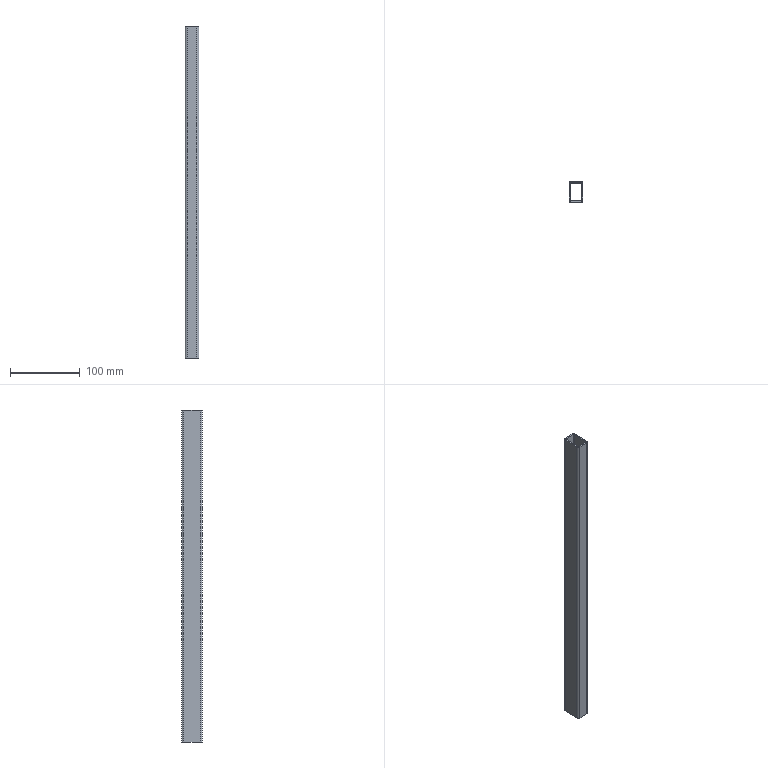Part | STEP file | DIN EN 10305-5 - 35 x 20 x 2  - 454 | 1 solid | 18 faces | box 20 x 30 x 475 mm | volume 84138 mm3 | plane 10 | cylinder 8 | commonest cylinder face diameters 2 x4 6 x4
STEP:
#1=CARTESIAN_POINT('',(0.,0.,0.));
#2=DIRECTION('',(0.,0.,1.));
#3=DIRECTION('',(1.,0.,0.));
#4=AXIS2_PLACEMENT_3D('',#1,#2,#3);
#5=CARTESIAN_POINT('',(-7.,-13.,475.));
#6=VERTEX_POINT('',#5);
#7=CARTESIAN_POINT('',(7.,-13.,475.));
#8=VERTEX_POINT('',#7);
#9=CARTESIAN_POINT('',(3.5,-13.,475.));
#10=DIRECTION('',(1.,0.,0.));
#11=VECTOR('',#10,1.);
#12=LINE('',#9,#11);
#13=CARTESIAN_POINT('',(7.,-13.,0.));
#14=DIRECTION('',(0.,-1.,0.));
#15=DIRECTION('',(0.,0.,-1.));
#16=AXIS2_PLACEMENT_3D('',#13,#14,#15);
#17=PLANE('',#16);
#18=CARTESIAN_POINT('',(-475.,-3.5));
#19=DIRECTION('',(0.,1.));
#20=VECTOR('',#19,1.);
#21=LINE('',#18,#20);
#22=(GEOMETRIC_REPRESENTATION_CONTEXT(2)PARAMETRIC_REPRESENTATION_CONTEXT()REPRESENTATION_CONTEXT('',''));
#23=DEFINITIONAL_REPRESENTATION('',(#21),#22);
#24=PCURVE('',#17,#23);
#25=CARTESIAN_POINT('',(0.,0.,475.));
#26=DIRECTION('',(0.,0.,1.));
#27=DIRECTION('',(1.,0.,0.));
#28=AXIS2_PLACEMENT_3D('',#25,#26,#27);
#29=PLANE('',#28);
#30=CARTESIAN_POINT('',(3.5,-13.));
#31=DIRECTION('',(1.,0.));
#32=VECTOR('',#31,1.);
#33=LINE('',#30,#32);
#34=(GEOMETRIC_REPRESENTATION_CONTEXT(2)PARAMETRIC_REPRESENTATION_CONTEXT()REPRESENTATION_CONTEXT('',''));
#35=DEFINITIONAL_REPRESENTATION('',(#33),#34);
#36=PCURVE('',#29,#35);
#37=SURFACE_CURVE('',#12,(#24,#36),.PCURVE_S1.);
#38=EDGE_CURVE('',#6,#8,#37,.T.);
#39=ORIENTED_EDGE('',*,*,#38,.T.);
#40=CARTESIAN_POINT('',(7.,-13.,0.));
#41=VERTEX_POINT('',#40);
#42=CARTESIAN_POINT('',(7.,-13.,0.));
#43=DIRECTION('',(0.,0.,1.));
#44=VECTOR('',#43,1.);
#45=LINE('',#42,#44);
#46=CARTESIAN_POINT('',(0.,0.));
#47=DIRECTION('',(-1.,0.));
#48=VECTOR('',#47,1.);
#49=LINE('',#46,#48);
#50=(GEOMETRIC_REPRESENTATION_CONTEXT(2)PARAMETRIC_REPRESENTATION_CONTEXT()REPRESENTATION_CONTEXT('',''));
#51=DEFINITIONAL_REPRESENTATION('',(#49),#50);
#52=PCURVE('',#17,#51);
#53=CARTESIAN_POINT('',(7.,-12.,0.));
#54=DIRECTION('',(0.,0.,1.));
#55=DIRECTION('',(0.,1.,0.));
#56=AXIS2_PLACEMENT_3D('',#53,#54,#55);
#57=CYLINDRICAL_SURFACE('',#56,1.);
#58=CARTESIAN_POINT('',(3.142,0.));
#59=DIRECTION('',(0.,1.));
#60=VECTOR('',#59,1.);
#61=LINE('',#58,#60);
#62=(GEOMETRIC_REPRESENTATION_CONTEXT(2)PARAMETRIC_REPRESENTATION_CONTEXT()REPRESENTATION_CONTEXT('',''));
#63=DEFINITIONAL_REPRESENTATION('',(#61),#62);
#64=PCURVE('',#57,#63);
#65=SURFACE_CURVE('',#45,(#52,#64),.PCURVE_S1.);
#66=EDGE_CURVE('',#41,#8,#65,.T.);
#67=ORIENTED_EDGE('',*,*,#66,.F.);
#68=CARTESIAN_POINT('',(-7.,-13.,0.));
#69=VERTEX_POINT('',#68);
#70=CARTESIAN_POINT('',(3.5,-13.,0.));
#71=DIRECTION('',(1.,0.,0.));
#72=VECTOR('',#71,1.);
#73=LINE('',#70,#72);
#74=CARTESIAN_POINT('',(0.,-3.5));
#75=DIRECTION('',(0.,1.));
#76=VECTOR('',#75,1.);
#77=LINE('',#74,#76);
#78=(GEOMETRIC_REPRESENTATION_CONTEXT(2)PARAMETRIC_REPRESENTATION_CONTEXT()REPRESENTATION_CONTEXT('',''));
#79=DEFINITIONAL_REPRESENTATION('',(#77),#78);
#80=PCURVE('',#17,#79);
#81=CARTESIAN_POINT('',(0.,0.,0.));
#82=DIRECTION('',(0.,0.,1.));
#83=DIRECTION('',(1.,0.,0.));
#84=AXIS2_PLACEMENT_3D('',#81,#82,#83);
#85=PLANE('',#84);
#86=CARTESIAN_POINT('',(3.5,-13.));
#87=DIRECTION('',(1.,0.));
#88=VECTOR('',#87,1.);
#89=LINE('',#86,#88);
#90=(GEOMETRIC_REPRESENTATION_CONTEXT(2)PARAMETRIC_REPRESENTATION_CONTEXT()REPRESENTATION_CONTEXT('',''));
#91=DEFINITIONAL_REPRESENTATION('',(#89),#90);
#92=PCURVE('',#85,#91);
#93=SURFACE_CURVE('',#73,(#80,#92),.PCURVE_S1.);
#94=EDGE_CURVE('',#69,#41,#93,.T.);
#95=ORIENTED_EDGE('',*,*,#94,.F.);
#96=CARTESIAN_POINT('',(-7.,-13.,0.));
#97=DIRECTION('',(0.,0.,1.));
#98=VECTOR('',#97,1.);
#99=LINE('',#96,#98);
#100=CARTESIAN_POINT('',(0.,-14.));
#101=DIRECTION('',(-1.,0.));
#102=VECTOR('',#101,1.);
#103=LINE('',#100,#102);
#104=(GEOMETRIC_REPRESENTATION_CONTEXT(2)PARAMETRIC_REPRESENTATION_CONTEXT()REPRESENTATION_CONTEXT('',''));
#105=DEFINITIONAL_REPRESENTATION('',(#103),#104);
#106=PCURVE('',#17,#105);
#107=CARTESIAN_POINT('',(-7.,-12.,0.));
#108=DIRECTION('',(0.,0.,1.));
#109=DIRECTION('',(1.,0.,0.));
#110=AXIS2_PLACEMENT_3D('',#107,#108,#109);
#111=CYLINDRICAL_SURFACE('',#110,1.);
#112=CARTESIAN_POINT('',(4.712,0.));
#113=DIRECTION('',(0.,1.));
#114=VECTOR('',#113,1.);
#115=LINE('',#112,#114);
#116=(GEOMETRIC_REPRESENTATION_CONTEXT(2)PARAMETRIC_REPRESENTATION_CONTEXT()REPRESENTATION_CONTEXT('',''));
#117=DEFINITIONAL_REPRESENTATION('',(#115),#116);
#118=PCURVE('',#111,#117);
#119=SURFACE_CURVE('',#99,(#106,#118),.PCURVE_S1.);
#120=EDGE_CURVE('',#69,#6,#119,.T.);
#121=ORIENTED_EDGE('',*,*,#120,.T.);
#122=EDGE_LOOP('',(#39,#67,#95,#121));
#123=FACE_BOUND('',#122,.T.);
#124=ADVANCED_FACE('',(#123),#17,.F.);
#125=ORIENTED_EDGE('',*,*,#66,.F.);
#126=CARTESIAN_POINT('',(8.,-12.,0.));
#127=VERTEX_POINT('',#126);
#128=CARTESIAN_POINT('',(7.,-12.,0.));
#129=DIRECTION('',(0.,0.,1.));
#130=DIRECTION('',(0.,1.,0.));
#131=AXIS2_PLACEMENT_3D('',#128,#129,#130);
#132=CIRCLE('',#131,1.);
#133=CARTESIAN_POINT('',(0.,0.));
#134=DIRECTION('',(1.,0.));
#135=VECTOR('',#134,1.);
#136=LINE('',#133,#135);
#137=(GEOMETRIC_REPRESENTATION_CONTEXT(2)PARAMETRIC_REPRESENTATION_CONTEXT()REPRESENTATION_CONTEXT('',''));
#138=DEFINITIONAL_REPRESENTATION('',(#136),#137);
#139=PCURVE('',#57,#138);
#140=CARTESIAN_POINT('',(7.,-12.));
#141=DIRECTION('',(0.,1.));
#142=AXIS2_PLACEMENT_2D('',#140,#141);
#143=CIRCLE('',#142,1.);
#144=(GEOMETRIC_REPRESENTATION_CONTEXT(2)PARAMETRIC_REPRESENTATION_CONTEXT()REPRESENTATION_CONTEXT('',''));
#145=DEFINITIONAL_REPRESENTATION('',(#143),#144);
#146=PCURVE('',#85,#145);
#147=SURFACE_CURVE('',#132,(#139,#146),.PCURVE_S1.);
#148=EDGE_CURVE('',#41,#127,#147,.T.);
#149=ORIENTED_EDGE('',*,*,#148,.T.);
#150=CARTESIAN_POINT('',(8.,-12.,475.));
#151=VERTEX_POINT('',#150);
#152=CARTESIAN_POINT('',(8.,-12.,0.));
#153=DIRECTION('',(0.,0.,1.));
#154=VECTOR('',#153,1.);
#155=LINE('',#152,#154);
#156=CARTESIAN_POINT('',(4.712,0.));
#157=DIRECTION('',(0.,1.));
#158=VECTOR('',#157,1.);
#159=LINE('',#156,#158);
#160=(GEOMETRIC_REPRESENTATION_CONTEXT(2)PARAMETRIC_REPRESENTATION_CONTEXT()REPRESENTATION_CONTEXT('',''));
#161=DEFINITIONAL_REPRESENTATION('',(#159),#160);
#162=PCURVE('',#57,#161);
#163=CARTESIAN_POINT('',(8.,12.,0.));
#164=DIRECTION('',(1.,0.,0.));
#165=DIRECTION('',(0.,0.,-1.));
#166=AXIS2_PLACEMENT_3D('',#163,#164,#165);
#167=PLANE('',#166);
#168=CARTESIAN_POINT('',(0.,-24.));
#169=DIRECTION('',(-1.,0.));
#170=VECTOR('',#169,1.);
#171=LINE('',#168,#170);
#172=(GEOMETRIC_REPRESENTATION_CONTEXT(2)PARAMETRIC_REPRESENTATION_CONTEXT()REPRESENTATION_CONTEXT('',''));
#173=DEFINITIONAL_REPRESENTATION('',(#171),#172);
#174=PCURVE('',#167,#173);
#175=SURFACE_CURVE('',#155,(#162,#174),.PCURVE_S1.);
#176=EDGE_CURVE('',#127,#151,#175,.T.);
#177=ORIENTED_EDGE('',*,*,#176,.T.);
#178=CARTESIAN_POINT('',(7.,-12.,475.));
#179=DIRECTION('',(0.,0.,1.));
#180=DIRECTION('',(0.,1.,0.));
#181=AXIS2_PLACEMENT_3D('',#178,#179,#180);
#182=CIRCLE('',#181,1.);
#183=CARTESIAN_POINT('',(0.,475.));
#184=DIRECTION('',(1.,0.));
#185=VECTOR('',#184,1.);
#186=LINE('',#183,#185);
#187=(GEOMETRIC_REPRESENTATION_CONTEXT(2)PARAMETRIC_REPRESENTATION_CONTEXT()REPRESENTATION_CONTEXT('',''));
#188=DEFINITIONAL_REPRESENTATION('',(#186),#187);
#189=PCURVE('',#57,#188);
#190=CARTESIAN_POINT('',(7.,-12.));
#191=DIRECTION('',(0.,1.));
#192=AXIS2_PLACEMENT_2D('',#190,#191);
#193=CIRCLE('',#192,1.);
#194=(GEOMETRIC_REPRESENTATION_CONTEXT(2)PARAMETRIC_REPRESENTATION_CONTEXT()REPRESENTATION_CONTEXT('',''));
#195=DEFINITIONAL_REPRESENTATION('',(#193),#194);
#196=PCURVE('',#29,#195);
#197=SURFACE_CURVE('',#182,(#189,#196),.PCURVE_S1.);
#198=EDGE_CURVE('',#8,#151,#197,.T.);
#199=ORIENTED_EDGE('',*,*,#198,.F.);
#200=EDGE_LOOP('',(#125,#149,#177,#199));
#201=FACE_BOUND('',#200,.F.);
#202=ADVANCED_FACE('',(#201),#57,.F.);
#203=CARTESIAN_POINT('',(8.,12.,475.));
#204=VERTEX_POINT('',#203);
#205=CARTESIAN_POINT('',(8.,6.,475.));
#206=DIRECTION('',(0.,1.,0.));
#207=VECTOR('',#206,1.);
#208=LINE('',#205,#207);
#209=CARTESIAN_POINT('',(-475.,-6.));
#210=DIRECTION('',(0.,1.));
#211=VECTOR('',#210,1.);
#212=LINE('',#209,#211);
#213=(GEOMETRIC_REPRESENTATION_CONTEXT(2)PARAMETRIC_REPRESENTATION_CONTEXT()REPRESENTATION_CONTEXT('',''));
#214=DEFINITIONAL_REPRESENTATION('',(#212),#213);
#215=PCURVE('',#167,#214);
#216=CARTESIAN_POINT('',(8.,6.));
#217=DIRECTION('',(0.,1.));
#218=VECTOR('',#217,1.);
#219=LINE('',#216,#218);
#220=(GEOMETRIC_REPRESENTATION_CONTEXT(2)PARAMETRIC_REPRESENTATION_CONTEXT()REPRESENTATION_CONTEXT('',''));
#221=DEFINITIONAL_REPRESENTATION('',(#219),#220);
#222=PCURVE('',#29,#221);
#223=SURFACE_CURVE('',#208,(#215,#222),.PCURVE_S1.);
#224=EDGE_CURVE('',#151,#204,#223,.T.);
#225=ORIENTED_EDGE('',*,*,#224,.T.);
#226=CARTESIAN_POINT('',(8.,12.,0.));
#227=VERTEX_POINT('',#226);
#228=CARTESIAN_POINT('',(8.,12.,0.));
#229=DIRECTION('',(0.,0.,1.));
#230=VECTOR('',#229,1.);
#231=LINE('',#228,#230);
#232=CARTESIAN_POINT('',(0.,0.));
#233=DIRECTION('',(-1.,0.));
#234=VECTOR('',#233,1.);
#235=LINE('',#232,#234);
#236=(GEOMETRIC_REPRESENTATION_CONTEXT(2)PARAMETRIC_REPRESENTATION_CONTEXT()REPRESENTATION_CONTEXT('',''));
#237=DEFINITIONAL_REPRESENTATION('',(#235),#236);
#238=PCURVE('',#167,#237);
#239=CARTESIAN_POINT('',(7.,12.,0.));
#240=DIRECTION('',(0.,0.,1.));
#241=DIRECTION('',(-1.,0.,0.));
#242=AXIS2_PLACEMENT_3D('',#239,#240,#241);
#243=CYLINDRICAL_SURFACE('',#242,1.);
#244=CARTESIAN_POINT('',(3.142,0.));
#245=DIRECTION('',(0.,1.));
#246=VECTOR('',#245,1.);
#247=LINE('',#244,#246);
#248=(GEOMETRIC_REPRESENTATION_CONTEXT(2)PARAMETRIC_REPRESENTATION_CONTEXT()REPRESENTATION_CONTEXT('',''));
#249=DEFINITIONAL_REPRESENTATION('',(#247),#248);
#250=PCURVE('',#243,#249);
#251=SURFACE_CURVE('',#231,(#238,#250),.PCURVE_S1.);
#252=EDGE_CURVE('',#227,#204,#251,.T.);
#253=ORIENTED_EDGE('',*,*,#252,.F.);
#254=CARTESIAN_POINT('',(8.,6.,0.));
#255=DIRECTION('',(0.,1.,0.));
#256=VECTOR('',#255,1.);
#257=LINE('',#254,#256);
#258=CARTESIAN_POINT('',(0.,-6.));
#259=DIRECTION('',(0.,1.));
#260=VECTOR('',#259,1.);
#261=LINE('',#258,#260);
#262=(GEOMETRIC_REPRESENTATION_CONTEXT(2)PARAMETRIC_REPRESENTATION_CONTEXT()REPRESENTATION_CONTEXT('',''));
#263=DEFINITIONAL_REPRESENTATION('',(#261),#262);
#264=PCURVE('',#167,#263);
#265=CARTESIAN_POINT('',(8.,6.));
#266=DIRECTION('',(0.,1.));
#267=VECTOR('',#266,1.);
#268=LINE('',#265,#267);
#269=(GEOMETRIC_REPRESENTATION_CONTEXT(2)PARAMETRIC_REPRESENTATION_CONTEXT()REPRESENTATION_CONTEXT('',''));
#270=DEFINITIONAL_REPRESENTATION('',(#268),#269);
#271=PCURVE('',#85,#270);
#272=SURFACE_CURVE('',#257,(#264,#271),.PCURVE_S1.);
#273=EDGE_CURVE('',#127,#227,#272,.T.);
#274=ORIENTED_EDGE('',*,*,#273,.F.);
#275=ORIENTED_EDGE('',*,*,#176,.T.);
#276=EDGE_LOOP('',(#225,#253,#274,#275));
#277=FACE_BOUND('',#276,.T.);
#278=ADVANCED_FACE('',(#277),#167,.F.);
#279=ORIENTED_EDGE('',*,*,#252,.F.);
#280=CARTESIAN_POINT('',(7.,13.,0.));
#281=VERTEX_POINT('',#280);
#282=CARTESIAN_POINT('',(7.,12.,0.));
#283=DIRECTION('',(0.,0.,1.));
#284=DIRECTION('',(-1.,0.,0.));
#285=AXIS2_PLACEMENT_3D('',#282,#283,#284);
#286=CIRCLE('',#285,1.);
#287=CARTESIAN_POINT('',(0.,0.));
#288=DIRECTION('',(1.,0.));
#289=VECTOR('',#288,1.);
#290=LINE('',#287,#289);
#291=(GEOMETRIC_REPRESENTATION_CONTEXT(2)PARAMETRIC_REPRESENTATION_CONTEXT()REPRESENTATION_CONTEXT('',''));
#292=DEFINITIONAL_REPRESENTATION('',(#290),#291);
#293=PCURVE('',#243,#292);
#294=CARTESIAN_POINT('',(7.,12.));
#295=DIRECTION('',(-1.,0.));
#296=AXIS2_PLACEMENT_2D('',#294,#295);
#297=CIRCLE('',#296,1.);
#298=(GEOMETRIC_REPRESENTATION_CONTEXT(2)PARAMETRIC_REPRESENTATION_CONTEXT()REPRESENTATION_CONTEXT('',''));
#299=DEFINITIONAL_REPRESENTATION('',(#297),#298);
#300=PCURVE('',#85,#299);
#301=SURFACE_CURVE('',#286,(#293,#300),.PCURVE_S1.);
#302=EDGE_CURVE('',#227,#281,#301,.T.);
#303=ORIENTED_EDGE('',*,*,#302,.T.);
#304=CARTESIAN_POINT('',(7.,13.,475.));
#305=VERTEX_POINT('',#304);
#306=CARTESIAN_POINT('',(7.,13.,0.));
#307=DIRECTION('',(0.,0.,1.));
#308=VECTOR('',#307,1.);
#309=LINE('',#306,#308);
#310=CARTESIAN_POINT('',(4.712,0.));
#311=DIRECTION('',(0.,1.));
#312=VECTOR('',#311,1.);
#313=LINE('',#310,#312);
#314=(GEOMETRIC_REPRESENTATION_CONTEXT(2)PARAMETRIC_REPRESENTATION_CONTEXT()REPRESENTATION_CONTEXT('',''));
#315=DEFINITIONAL_REPRESENTATION('',(#313),#314);
#316=PCURVE('',#243,#315);
#317=CARTESIAN_POINT('',(-7.,13.,0.));
#318=DIRECTION('',(0.,1.,0.));
#319=DIRECTION('',(0.,0.,1.));
#320=AXIS2_PLACEMENT_3D('',#317,#318,#319);
#321=PLANE('',#320);
#322=CARTESIAN_POINT('',(0.,14.));
#323=DIRECTION('',(1.,0.));
#324=VECTOR('',#323,1.);
#325=LINE('',#322,#324);
#326=(GEOMETRIC_REPRESENTATION_CONTEXT(2)PARAMETRIC_REPRESENTATION_CONTEXT()REPRESENTATION_CONTEXT('',''));
#327=DEFINITIONAL_REPRESENTATION('',(#325),#326);
#328=PCURVE('',#321,#327);
#329=SURFACE_CURVE('',#309,(#316,#328),.PCURVE_S1.);
#330=EDGE_CURVE('',#281,#305,#329,.T.);
#331=ORIENTED_EDGE('',*,*,#330,.T.);
#332=CARTESIAN_POINT('',(7.,12.,475.));
#333=DIRECTION('',(0.,0.,1.));
#334=DIRECTION('',(-1.,0.,0.));
#335=AXIS2_PLACEMENT_3D('',#332,#333,#334);
#336=CIRCLE('',#335,1.);
#337=CARTESIAN_POINT('',(0.,475.));
#338=DIRECTION('',(1.,0.));
#339=VECTOR('',#338,1.);
#340=LINE('',#337,#339);
#341=(GEOMETRIC_REPRESENTATION_CONTEXT(2)PARAMETRIC_REPRESENTATION_CONTEXT()REPRESENTATION_CONTEXT('',''));
#342=DEFINITIONAL_REPRESENTATION('',(#340),#341);
#343=PCURVE('',#243,#342);
#344=CARTESIAN_POINT('',(7.,12.));
#345=DIRECTION('',(-1.,0.));
#346=AXIS2_PLACEMENT_2D('',#344,#345);
#347=CIRCLE('',#346,1.);
#348=(GEOMETRIC_REPRESENTATION_CONTEXT(2)PARAMETRIC_REPRESENTATION_CONTEXT()REPRESENTATION_CONTEXT('',''));
#349=DEFINITIONAL_REPRESENTATION('',(#347),#348);
#350=PCURVE('',#29,#349);
#351=SURFACE_CURVE('',#336,(#343,#350),.PCURVE_S1.);
#352=EDGE_CURVE('',#204,#305,#351,.T.);
#353=ORIENTED_EDGE('',*,*,#352,.F.);
#354=EDGE_LOOP('',(#279,#303,#331,#353));
#355=FACE_BOUND('',#354,.F.);
#356=ADVANCED_FACE('',(#355),#243,.F.);
#357=CARTESIAN_POINT('',(10.,12.,475.));
#358=VERTEX_POINT('',#357);
#359=CARTESIAN_POINT('',(10.,-12.,475.));
#360=VERTEX_POINT('',#359);
#361=CARTESIAN_POINT('',(10.,6.,475.));
#362=DIRECTION('',(0.,-1.,0.));
#363=VECTOR('',#362,1.);
#364=LINE('',#361,#363);
#365=CARTESIAN_POINT('',(10.,12.,0.));
#366=DIRECTION('',(1.,0.,0.));
#367=DIRECTION('',(0.,0.,-1.));
#368=AXIS2_PLACEMENT_3D('',#365,#366,#367);
#369=PLANE('',#368);
#370=CARTESIAN_POINT('',(-475.,-6.));
#371=DIRECTION('',(0.,-1.));
#372=VECTOR('',#371,1.);
#373=LINE('',#370,#372);
#374=(GEOMETRIC_REPRESENTATION_CONTEXT(2)PARAMETRIC_REPRESENTATION_CONTEXT()REPRESENTATION_CONTEXT('',''));
#375=DEFINITIONAL_REPRESENTATION('',(#373),#374);
#376=PCURVE('',#369,#375);
#377=CARTESIAN_POINT('',(10.,6.));
#378=DIRECTION('',(0.,-1.));
#379=VECTOR('',#378,1.);
#380=LINE('',#377,#379);
#381=(GEOMETRIC_REPRESENTATION_CONTEXT(2)PARAMETRIC_REPRESENTATION_CONTEXT()REPRESENTATION_CONTEXT('',''));
#382=DEFINITIONAL_REPRESENTATION('',(#380),#381);
#383=PCURVE('',#29,#382);
#384=SURFACE_CURVE('',#364,(#376,#383),.PCURVE_S1.);
#385=EDGE_CURVE('',#358,#360,#384,.T.);
#386=ORIENTED_EDGE('',*,*,#385,.T.);
#387=CARTESIAN_POINT('',(10.,-12.,0.));
#388=VERTEX_POINT('',#387);
#389=CARTESIAN_POINT('',(10.,-12.,0.));
#390=DIRECTION('',(0.,0.,1.));
#391=VECTOR('',#390,1.);
#392=LINE('',#389,#391);
#393=CARTESIAN_POINT('',(0.,-24.));
#394=DIRECTION('',(-1.,0.));
#395=VECTOR('',#394,1.);
#396=LINE('',#393,#395);
#397=(GEOMETRIC_REPRESENTATION_CONTEXT(2)PARAMETRIC_REPRESENTATION_CONTEXT()REPRESENTATION_CONTEXT('',''));
#398=DEFINITIONAL_REPRESENTATION('',(#396),#397);
#399=PCURVE('',#369,#398);
#400=CARTESIAN_POINT('',(7.,-12.,0.));
#401=DIRECTION('',(0.,0.,1.));
#402=DIRECTION('',(0.,1.,0.));
#403=AXIS2_PLACEMENT_3D('',#400,#401,#402);
#404=CYLINDRICAL_SURFACE('',#403,3.);
#405=CARTESIAN_POINT('',(4.712,0.));
#406=DIRECTION('',(0.,1.));
#407=VECTOR('',#406,1.);
#408=LINE('',#405,#407);
#409=(GEOMETRIC_REPRESENTATION_CONTEXT(2)PARAMETRIC_REPRESENTATION_CONTEXT()REPRESENTATION_CONTEXT('',''));
#410=DEFINITIONAL_REPRESENTATION('',(#408),#409);
#411=PCURVE('',#404,#410);
#412=SURFACE_CURVE('',#392,(#399,#411),.PCURVE_S1.);
#413=EDGE_CURVE('',#388,#360,#412,.T.);
#414=ORIENTED_EDGE('',*,*,#413,.F.);
#415=CARTESIAN_POINT('',(10.,12.,0.));
#416=VERTEX_POINT('',#415);
#417=CARTESIAN_POINT('',(10.,6.,0.));
#418=DIRECTION('',(0.,-1.,0.));
#419=VECTOR('',#418,1.);
#420=LINE('',#417,#419);
#421=CARTESIAN_POINT('',(0.,-6.));
#422=DIRECTION('',(0.,-1.));
#423=VECTOR('',#422,1.);
#424=LINE('',#421,#423);
#425=(GEOMETRIC_REPRESENTATION_CONTEXT(2)PARAMETRIC_REPRESENTATION_CONTEXT()REPRESENTATION_CONTEXT('',''));
#426=DEFINITIONAL_REPRESENTATION('',(#424),#425);
#427=PCURVE('',#369,#426);
#428=CARTESIAN_POINT('',(10.,6.));
#429=DIRECTION('',(0.,-1.));
#430=VECTOR('',#429,1.);
#431=LINE('',#428,#430);
#432=(GEOMETRIC_REPRESENTATION_CONTEXT(2)PARAMETRIC_REPRESENTATION_CONTEXT()REPRESENTATION_CONTEXT('',''));
#433=DEFINITIONAL_REPRESENTATION('',(#431),#432);
#434=PCURVE('',#85,#433);
#435=SURFACE_CURVE('',#420,(#427,#434),.PCURVE_S1.);
#436=EDGE_CURVE('',#416,#388,#435,.T.);
#437=ORIENTED_EDGE('',*,*,#436,.F.);
#438=CARTESIAN_POINT('',(10.,12.,0.));
#439=DIRECTION('',(0.,0.,1.));
#440=VECTOR('',#439,1.);
#441=LINE('',#438,#440);
#442=CARTESIAN_POINT('',(0.,0.));
#443=DIRECTION('',(-1.,0.));
#444=VECTOR('',#443,1.);
#445=LINE('',#442,#444);
#446=(GEOMETRIC_REPRESENTATION_CONTEXT(2)PARAMETRIC_REPRESENTATION_CONTEXT()REPRESENTATION_CONTEXT('',''));
#447=DEFINITIONAL_REPRESENTATION('',(#445),#446);
#448=PCURVE('',#369,#447);
#449=CARTESIAN_POINT('',(7.,12.,0.));
#450=DIRECTION('',(0.,0.,1.));
#451=DIRECTION('',(-1.,0.,0.));
#452=AXIS2_PLACEMENT_3D('',#449,#450,#451);
#453=CYLINDRICAL_SURFACE('',#452,3.);
#454=CARTESIAN_POINT('',(3.142,0.));
#455=DIRECTION('',(0.,1.));
#456=VECTOR('',#455,1.);
#457=LINE('',#454,#456);
#458=(GEOMETRIC_REPRESENTATION_CONTEXT(2)PARAMETRIC_REPRESENTATION_CONTEXT()REPRESENTATION_CONTEXT('',''));
#459=DEFINITIONAL_REPRESENTATION('',(#457),#458);
#460=PCURVE('',#453,#459);
#461=SURFACE_CURVE('',#441,(#448,#460),.PCURVE_S1.);
#462=EDGE_CURVE('',#416,#358,#461,.T.);
#463=ORIENTED_EDGE('',*,*,#462,.T.);
#464=EDGE_LOOP('',(#386,#414,#437,#463));
#465=FACE_BOUND('',#464,.T.);
#466=ADVANCED_FACE('',(#465),#369,.T.);
#467=CARTESIAN_POINT('',(7.,-15.,475.));
#468=VERTEX_POINT('',#467);
#469=CARTESIAN_POINT('',(7.,-12.,475.));
#470=DIRECTION('',(0.,0.,-1.));
#471=DIRECTION('',(0.,1.,0.));
#472=AXIS2_PLACEMENT_3D('',#469,#470,#471);
#473=CIRCLE('',#472,3.);
#474=CARTESIAN_POINT('',(6.283,475.));
#475=DIRECTION('',(-1.,0.));
#476=VECTOR('',#475,1.);
#477=LINE('',#474,#476);
#478=(GEOMETRIC_REPRESENTATION_CONTEXT(2)PARAMETRIC_REPRESENTATION_CONTEXT()REPRESENTATION_CONTEXT('',''));
#479=DEFINITIONAL_REPRESENTATION('',(#477),#478);
#480=PCURVE('',#404,#479);
#481=CARTESIAN_POINT('',(7.,-9.));
#482=CARTESIAN_POINT('',(12.196,-9.));
#483=CARTESIAN_POINT('',(9.598,-13.5));
#484=CARTESIAN_POINT('',(7.,-18.));
#485=CARTESIAN_POINT('',(4.402,-13.5));
#486=CARTESIAN_POINT('',(1.804,-9.));
#487=CARTESIAN_POINT('',(7.,-9.));
#488=(BOUNDED_CURVE()B_SPLINE_CURVE(2,(#481,#482,#483,#484,#485,#486,#487),.UNSPECIFIED.,.T.,.F.)B_SPLINE_CURVE_WITH_KNOTS((1,2,2,2,2,1),(-2.094,0.,2.094,4.189,6.283,8.378),.UNSPECIFIED.)CURVE()GEOMETRIC_REPRESENTATION_ITEM()RATIONAL_B_SPLINE_CURVE((1.,0.5,1.,0.5,1.,0.5,1.))REPRESENTATION_ITEM(''));
#489=(GEOMETRIC_REPRESENTATION_CONTEXT(2)PARAMETRIC_REPRESENTATION_CONTEXT()REPRESENTATION_CONTEXT('',''));
#490=DEFINITIONAL_REPRESENTATION('',(#488),#489);
#491=PCURVE('',#29,#490);
#492=SURFACE_CURVE('',#473,(#480,#491),.PCURVE_S1.);
#493=EDGE_CURVE('',#360,#468,#492,.T.);
#494=ORIENTED_EDGE('',*,*,#493,.T.);
#495=CARTESIAN_POINT('',(7.,-15.,0.));
#496=VERTEX_POINT('',#495);
#497=CARTESIAN_POINT('',(7.,-15.,0.));
#498=DIRECTION('',(0.,0.,1.));
#499=VECTOR('',#498,1.);
#500=LINE('',#497,#499);
#501=CARTESIAN_POINT('',(3.142,0.));
#502=DIRECTION('',(0.,1.));
#503=VECTOR('',#502,1.);
#504=LINE('',#501,#503);
#505=(GEOMETRIC_REPRESENTATION_CONTEXT(2)PARAMETRIC_REPRESENTATION_CONTEXT()REPRESENTATION_CONTEXT('',''));
#506=DEFINITIONAL_REPRESENTATION('',(#504),#505);
#507=PCURVE('',#404,#506);
#508=CARTESIAN_POINT('',(7.,-15.,0.));
#509=DIRECTION('',(0.,-1.,0.));
#510=DIRECTION('',(0.,0.,-1.));
#511=AXIS2_PLACEMENT_3D('',#508,#509,#510);
#512=PLANE('',#511);
#513=CARTESIAN_POINT('',(0.,0.));
#514=DIRECTION('',(-1.,0.));
#515=VECTOR('',#514,1.);
#516=LINE('',#513,#515);
#517=(GEOMETRIC_REPRESENTATION_CONTEXT(2)PARAMETRIC_REPRESENTATION_CONTEXT()REPRESENTATION_CONTEXT('',''));
#518=DEFINITIONAL_REPRESENTATION('',(#516),#517);
#519=PCURVE('',#512,#518);
#520=SURFACE_CURVE('',#500,(#507,#519),.PCURVE_S1.);
#521=EDGE_CURVE('',#496,#468,#520,.T.);
#522=ORIENTED_EDGE('',*,*,#521,.F.);
#523=CARTESIAN_POINT('',(7.,-12.,0.));
#524=DIRECTION('',(0.,0.,-1.));
#525=DIRECTION('',(0.,1.,0.));
#526=AXIS2_PLACEMENT_3D('',#523,#524,#525);
#527=CIRCLE('',#526,3.);
#528=CARTESIAN_POINT('',(6.283,0.));
#529=DIRECTION('',(-1.,0.));
#530=VECTOR('',#529,1.);
#531=LINE('',#528,#530);
#532=(GEOMETRIC_REPRESENTATION_CONTEXT(2)PARAMETRIC_REPRESENTATION_CONTEXT()REPRESENTATION_CONTEXT('',''));
#533=DEFINITIONAL_REPRESENTATION('',(#531),#532);
#534=PCURVE('',#404,#533);
#535=CARTESIAN_POINT('',(7.,-9.));
#536=CARTESIAN_POINT('',(12.196,-9.));
#537=CARTESIAN_POINT('',(9.598,-13.5));
#538=CARTESIAN_POINT('',(7.,-18.));
#539=CARTESIAN_POINT('',(4.402,-13.5));
#540=CARTESIAN_POINT('',(1.804,-9.));
#541=CARTESIAN_POINT('',(7.,-9.));
#542=(BOUNDED_CURVE()B_SPLINE_CURVE(2,(#535,#536,#537,#538,#539,#540,#541),.UNSPECIFIED.,.T.,.F.)B_SPLINE_CURVE_WITH_KNOTS((1,2,2,2,2,1),(-2.094,0.,2.094,4.189,6.283,8.378),.UNSPECIFIED.)CURVE()GEOMETRIC_REPRESENTATION_ITEM()RATIONAL_B_SPLINE_CURVE((1.,0.5,1.,0.5,1.,0.5,1.))REPRESENTATION_ITEM(''));
#543=(GEOMETRIC_REPRESENTATION_CONTEXT(2)PARAMETRIC_REPRESENTATION_CONTEXT()REPRESENTATION_CONTEXT('',''));
#544=DEFINITIONAL_REPRESENTATION('',(#542),#543);
#545=PCURVE('',#85,#544);
#546=SURFACE_CURVE('',#527,(#534,#545),.PCURVE_S1.);
#547=EDGE_CURVE('',#388,#496,#546,.T.);
#548=ORIENTED_EDGE('',*,*,#547,.F.);
#549=ORIENTED_EDGE('',*,*,#413,.T.);
#550=EDGE_LOOP('',(#494,#522,#548,#549));
#551=FACE_BOUND('',#550,.T.);
#552=ADVANCED_FACE('',(#551),#404,.T.);
#553=CARTESIAN_POINT('',(-7.,-15.,475.));
#554=VERTEX_POINT('',#553);
#555=CARTESIAN_POINT('',(3.5,-15.,475.));
#556=DIRECTION('',(-1.,0.,0.));
#557=VECTOR('',#556,1.);
#558=LINE('',#555,#557);
#559=CARTESIAN_POINT('',(-475.,-3.5));
#560=DIRECTION('',(0.,-1.));
#561=VECTOR('',#560,1.);
#562=LINE('',#559,#561);
#563=(GEOMETRIC_REPRESENTATION_CONTEXT(2)PARAMETRIC_REPRESENTATION_CONTEXT()REPRESENTATION_CONTEXT('',''));
#564=DEFINITIONAL_REPRESENTATION('',(#562),#563);
#565=PCURVE('',#512,#564);
#566=CARTESIAN_POINT('',(3.5,-15.));
#567=DIRECTION('',(-1.,0.));
#568=VECTOR('',#567,1.);
#569=LINE('',#566,#568);
#570=(GEOMETRIC_REPRESENTATION_CONTEXT(2)PARAMETRIC_REPRESENTATION_CONTEXT()REPRESENTATION_CONTEXT('',''));
#571=DEFINITIONAL_REPRESENTATION('',(#569),#570);
#572=PCURVE('',#29,#571);
#573=SURFACE_CURVE('',#558,(#565,#572),.PCURVE_S1.);
#574=EDGE_CURVE('',#468,#554,#573,.T.);
#575=ORIENTED_EDGE('',*,*,#574,.T.);
#576=CARTESIAN_POINT('',(-7.,-15.,0.));
#577=VERTEX_POINT('',#576);
#578=CARTESIAN_POINT('',(-7.,-15.,0.));
#579=DIRECTION('',(0.,0.,1.));
#580=VECTOR('',#579,1.);
#581=LINE('',#578,#580);
#582=CARTESIAN_POINT('',(0.,-14.));
#583=DIRECTION('',(-1.,0.));
#584=VECTOR('',#583,1.);
#585=LINE('',#582,#584);
#586=(GEOMETRIC_REPRESENTATION_CONTEXT(2)PARAMETRIC_REPRESENTATION_CONTEXT()REPRESENTATION_CONTEXT('',''));
#587=DEFINITIONAL_REPRESENTATION('',(#585),#586);
#588=PCURVE('',#512,#587);
#589=CARTESIAN_POINT('',(-7.,-12.,0.));
#590=DIRECTION('',(0.,0.,1.));
#591=DIRECTION('',(1.,0.,0.));
#592=AXIS2_PLACEMENT_3D('',#589,#590,#591);
#593=CYLINDRICAL_SURFACE('',#592,3.);
#594=CARTESIAN_POINT('',(4.712,0.));
#595=DIRECTION('',(0.,1.));
#596=VECTOR('',#595,1.);
#597=LINE('',#594,#596);
#598=(GEOMETRIC_REPRESENTATION_CONTEXT(2)PARAMETRIC_REPRESENTATION_CONTEXT()REPRESENTATION_CONTEXT('',''));
#599=DEFINITIONAL_REPRESENTATION('',(#597),#598);
#600=PCURVE('',#593,#599);
#601=SURFACE_CURVE('',#581,(#588,#600),.PCURVE_S1.);
#602=EDGE_CURVE('',#577,#554,#601,.T.);
#603=ORIENTED_EDGE('',*,*,#602,.F.);
#604=CARTESIAN_POINT('',(3.5,-15.,0.));
#605=DIRECTION('',(-1.,0.,0.));
#606=VECTOR('',#605,1.);
#607=LINE('',#604,#606);
#608=CARTESIAN_POINT('',(0.,-3.5));
#609=DIRECTION('',(0.,-1.));
#610=VECTOR('',#609,1.);
#611=LINE('',#608,#610);
#612=(GEOMETRIC_REPRESENTATION_CONTEXT(2)PARAMETRIC_REPRESENTATION_CONTEXT()REPRESENTATION_CONTEXT('',''));
#613=DEFINITIONAL_REPRESENTATION('',(#611),#612);
#614=PCURVE('',#512,#613);
#615=CARTESIAN_POINT('',(3.5,-15.));
#616=DIRECTION('',(-1.,0.));
#617=VECTOR('',#616,1.);
#618=LINE('',#615,#617);
#619=(GEOMETRIC_REPRESENTATION_CONTEXT(2)PARAMETRIC_REPRESENTATION_CONTEXT()REPRESENTATION_CONTEXT('',''));
#620=DEFINITIONAL_REPRESENTATION('',(#618),#619);
#621=PCURVE('',#85,#620);
#622=SURFACE_CURVE('',#607,(#614,#621),.PCURVE_S1.);
#623=EDGE_CURVE('',#496,#577,#622,.T.);
#624=ORIENTED_EDGE('',*,*,#623,.F.);
#625=ORIENTED_EDGE('',*,*,#521,.T.);
#626=EDGE_LOOP('',(#575,#603,#624,#625));
#627=FACE_BOUND('',#626,.T.);
#628=ADVANCED_FACE('',(#627),#512,.T.);
#629=CARTESIAN_POINT('',(-10.,-12.,475.));
#630=VERTEX_POINT('',#629);
#631=CARTESIAN_POINT('',(-7.,-12.,475.));
#632=DIRECTION('',(0.,0.,-1.));
#633=DIRECTION('',(1.,0.,0.));
#634=AXIS2_PLACEMENT_3D('',#631,#632,#633);
#635=CIRCLE('',#634,3.);
#636=CARTESIAN_POINT('',(6.283,475.));
#637=DIRECTION('',(-1.,0.));
#638=VECTOR('',#637,1.);
#639=LINE('',#636,#638);
#640=(GEOMETRIC_REPRESENTATION_CONTEXT(2)PARAMETRIC_REPRESENTATION_CONTEXT()REPRESENTATION_CONTEXT('',''));
#641=DEFINITIONAL_REPRESENTATION('',(#639),#640);
#642=PCURVE('',#593,#641);
#643=CARTESIAN_POINT('',(-4.,-12.));
#644=CARTESIAN_POINT('',(-4.,-17.196));
#645=CARTESIAN_POINT('',(-8.5,-14.598));
#646=CARTESIAN_POINT('',(-13.,-12.));
#647=CARTESIAN_POINT('',(-8.5,-9.402));
#648=CARTESIAN_POINT('',(-4.,-6.804));
#649=CARTESIAN_POINT('',(-4.,-12.));
#650=(BOUNDED_CURVE()B_SPLINE_CURVE(2,(#643,#644,#645,#646,#647,#648,#649),.UNSPECIFIED.,.T.,.F.)B_SPLINE_CURVE_WITH_KNOTS((1,2,2,2,2,1),(-2.094,0.,2.094,4.189,6.283,8.378),.UNSPECIFIED.)CURVE()GEOMETRIC_REPRESENTATION_ITEM()RATIONAL_B_SPLINE_CURVE((1.,0.5,1.,0.5,1.,0.5,1.))REPRESENTATION_ITEM(''));
#651=(GEOMETRIC_REPRESENTATION_CONTEXT(2)PARAMETRIC_REPRESENTATION_CONTEXT()REPRESENTATION_CONTEXT('',''));
#652=DEFINITIONAL_REPRESENTATION('',(#650),#651);
#653=PCURVE('',#29,#652);
#654=SURFACE_CURVE('',#635,(#642,#653),.PCURVE_S1.);
#655=EDGE_CURVE('',#554,#630,#654,.T.);
#656=ORIENTED_EDGE('',*,*,#655,.T.);
#657=CARTESIAN_POINT('',(-10.,-12.,0.));
#658=VERTEX_POINT('',#657);
#659=CARTESIAN_POINT('',(-10.,-12.,0.));
#660=DIRECTION('',(0.,0.,1.));
#661=VECTOR('',#660,1.);
#662=LINE('',#659,#661);
#663=CARTESIAN_POINT('',(3.142,0.));
#664=DIRECTION('',(0.,1.));
#665=VECTOR('',#664,1.);
#666=LINE('',#663,#665);
#667=(GEOMETRIC_REPRESENTATION_CONTEXT(2)PARAMETRIC_REPRESENTATION_CONTEXT()REPRESENTATION_CONTEXT('',''));
#668=DEFINITIONAL_REPRESENTATION('',(#666),#667);
#669=PCURVE('',#593,#668);
#670=CARTESIAN_POINT('',(-10.,-12.,0.));
#671=DIRECTION('',(-1.,0.,0.));
#672=DIRECTION('',(0.,0.,1.));
#673=AXIS2_PLACEMENT_3D('',#670,#671,#672);
#674=PLANE('',#673);
#675=CARTESIAN_POINT('',(0.,0.));
#676=DIRECTION('',(1.,0.));
#677=VECTOR('',#676,1.);
#678=LINE('',#675,#677);
#679=(GEOMETRIC_REPRESENTATION_CONTEXT(2)PARAMETRIC_REPRESENTATION_CONTEXT()REPRESENTATION_CONTEXT('',''));
#680=DEFINITIONAL_REPRESENTATION('',(#678),#679);
#681=PCURVE('',#674,#680);
#682=SURFACE_CURVE('',#662,(#669,#681),.PCURVE_S1.);
#683=EDGE_CURVE('',#658,#630,#682,.T.);
#684=ORIENTED_EDGE('',*,*,#683,.F.);
#685=CARTESIAN_POINT('',(-7.,-12.,0.));
#686=DIRECTION('',(0.,0.,-1.));
#687=DIRECTION('',(1.,0.,0.));
#688=AXIS2_PLACEMENT_3D('',#685,#686,#687);
#689=CIRCLE('',#688,3.);
#690=CARTESIAN_POINT('',(6.283,0.));
#691=DIRECTION('',(-1.,0.));
#692=VECTOR('',#691,1.);
#693=LINE('',#690,#692);
#694=(GEOMETRIC_REPRESENTATION_CONTEXT(2)PARAMETRIC_REPRESENTATION_CONTEXT()REPRESENTATION_CONTEXT('',''));
#695=DEFINITIONAL_REPRESENTATION('',(#693),#694);
#696=PCURVE('',#593,#695);
#697=CARTESIAN_POINT('',(-4.,-12.));
#698=CARTESIAN_POINT('',(-4.,-17.196));
#699=CARTESIAN_POINT('',(-8.5,-14.598));
#700=CARTESIAN_POINT('',(-13.,-12.));
#701=CARTESIAN_POINT('',(-8.5,-9.402));
#702=CARTESIAN_POINT('',(-4.,-6.804));
#703=CARTESIAN_POINT('',(-4.,-12.));
#704=(BOUNDED_CURVE()B_SPLINE_CURVE(2,(#697,#698,#699,#700,#701,#702,#703),.UNSPECIFIED.,.T.,.F.)B_SPLINE_CURVE_WITH_KNOTS((1,2,2,2,2,1),(-2.094,0.,2.094,4.189,6.283,8.378),.UNSPECIFIED.)CURVE()GEOMETRIC_REPRESENTATION_ITEM()RATIONAL_B_SPLINE_CURVE((1.,0.5,1.,0.5,1.,0.5,1.))REPRESENTATION_ITEM(''));
#705=(GEOMETRIC_REPRESENTATION_CONTEXT(2)PARAMETRIC_REPRESENTATION_CONTEXT()REPRESENTATION_CONTEXT('',''));
#706=DEFINITIONAL_REPRESENTATION('',(#704),#705);
#707=PCURVE('',#85,#706);
#708=SURFACE_CURVE('',#689,(#696,#707),.PCURVE_S1.);
#709=EDGE_CURVE('',#577,#658,#708,.T.);
#710=ORIENTED_EDGE('',*,*,#709,.F.);
#711=ORIENTED_EDGE('',*,*,#602,.T.);
#712=EDGE_LOOP('',(#656,#684,#710,#711));
#713=FACE_BOUND('',#712,.T.);
#714=ADVANCED_FACE('',(#713),#593,.T.);
#715=CARTESIAN_POINT('',(-7.,13.,475.));
#716=VERTEX_POINT('',#715);
#717=CARTESIAN_POINT('',(-3.5,13.,475.));
#718=DIRECTION('',(-1.,0.,0.));
#719=VECTOR('',#718,1.);
#720=LINE('',#717,#719);
#721=CARTESIAN_POINT('',(475.,3.5));
#722=DIRECTION('',(0.,-1.));
#723=VECTOR('',#722,1.);
#724=LINE('',#721,#723);
#725=(GEOMETRIC_REPRESENTATION_CONTEXT(2)PARAMETRIC_REPRESENTATION_CONTEXT()REPRESENTATION_CONTEXT('',''));
#726=DEFINITIONAL_REPRESENTATION('',(#724),#725);
#727=PCURVE('',#321,#726);
#728=CARTESIAN_POINT('',(-3.5,13.));
#729=DIRECTION('',(-1.,0.));
#730=VECTOR('',#729,1.);
#731=LINE('',#728,#730);
#732=(GEOMETRIC_REPRESENTATION_CONTEXT(2)PARAMETRIC_REPRESENTATION_CONTEXT()REPRESENTATION_CONTEXT('',''));
#733=DEFINITIONAL_REPRESENTATION('',(#731),#732);
#734=PCURVE('',#29,#733);
#735=SURFACE_CURVE('',#720,(#727,#734),.PCURVE_S1.);
#736=EDGE_CURVE('',#305,#716,#735,.T.);
#737=ORIENTED_EDGE('',*,*,#736,.T.);
#738=CARTESIAN_POINT('',(-7.,13.,0.));
#739=VERTEX_POINT('',#738);
#740=CARTESIAN_POINT('',(-7.,13.,0.));
#741=DIRECTION('',(0.,0.,1.));
#742=VECTOR('',#741,1.);
#743=LINE('',#740,#742);
#744=CARTESIAN_POINT('',(0.,0.));
#745=DIRECTION('',(1.,0.));
#746=VECTOR('',#745,1.);
#747=LINE('',#744,#746);
#748=(GEOMETRIC_REPRESENTATION_CONTEXT(2)PARAMETRIC_REPRESENTATION_CONTEXT()REPRESENTATION_CONTEXT('',''));
#749=DEFINITIONAL_REPRESENTATION('',(#747),#748);
#750=PCURVE('',#321,#749);
#751=CARTESIAN_POINT('',(-7.,12.,0.));
#752=DIRECTION('',(0.,0.,1.));
#753=DIRECTION('',(0.,-1.,0.));
#754=AXIS2_PLACEMENT_3D('',#751,#752,#753);
#755=CYLINDRICAL_SURFACE('',#754,1.);
#756=CARTESIAN_POINT('',(3.142,0.));
#757=DIRECTION('',(0.,1.));
#758=VECTOR('',#757,1.);
#759=LINE('',#756,#758);
#760=(GEOMETRIC_REPRESENTATION_CONTEXT(2)PARAMETRIC_REPRESENTATION_CONTEXT()REPRESENTATION_CONTEXT('',''));
#761=DEFINITIONAL_REPRESENTATION('',(#759),#760);
#762=PCURVE('',#755,#761);
#763=SURFACE_CURVE('',#743,(#750,#762),.PCURVE_S1.);
#764=EDGE_CURVE('',#739,#716,#763,.T.);
#765=ORIENTED_EDGE('',*,*,#764,.F.);
#766=CARTESIAN_POINT('',(-3.5,13.,0.));
#767=DIRECTION('',(-1.,0.,0.));
#768=VECTOR('',#767,1.);
#769=LINE('',#766,#768);
#770=CARTESIAN_POINT('',(0.,3.5));
#771=DIRECTION('',(0.,-1.));
#772=VECTOR('',#771,1.);
#773=LINE('',#770,#772);
#774=(GEOMETRIC_REPRESENTATION_CONTEXT(2)PARAMETRIC_REPRESENTATION_CONTEXT()REPRESENTATION_CONTEXT('',''));
#775=DEFINITIONAL_REPRESENTATION('',(#773),#774);
#776=PCURVE('',#321,#775);
#777=CARTESIAN_POINT('',(-3.5,13.));
#778=DIRECTION('',(-1.,0.));
#779=VECTOR('',#778,1.);
#780=LINE('',#777,#779);
#781=(GEOMETRIC_REPRESENTATION_CONTEXT(2)PARAMETRIC_REPRESENTATION_CONTEXT()REPRESENTATION_CONTEXT('',''));
#782=DEFINITIONAL_REPRESENTATION('',(#780),#781);
#783=PCURVE('',#85,#782);
#784=SURFACE_CURVE('',#769,(#776,#783),.PCURVE_S1.);
#785=EDGE_CURVE('',#281,#739,#784,.T.);
#786=ORIENTED_EDGE('',*,*,#785,.F.);
#787=ORIENTED_EDGE('',*,*,#330,.T.);
#788=EDGE_LOOP('',(#737,#765,#786,#787));
#789=FACE_BOUND('',#788,.T.);
#790=ADVANCED_FACE('',(#789),#321,.F.);
#791=CARTESIAN_POINT('',(-8.,-12.,0.));
#792=VERTEX_POINT('',#791);
#793=CARTESIAN_POINT('',(-8.,-12.,475.));
#794=VERTEX_POINT('',#793);
#795=CARTESIAN_POINT('',(-8.,-12.,0.));
#796=DIRECTION('',(0.,0.,1.));
#797=VECTOR('',#796,1.);
#798=LINE('',#795,#797);
#799=CARTESIAN_POINT('',(3.142,0.));
#800=DIRECTION('',(0.,1.));
#801=VECTOR('',#800,1.);
#802=LINE('',#799,#801);
#803=(GEOMETRIC_REPRESENTATION_CONTEXT(2)PARAMETRIC_REPRESENTATION_CONTEXT()REPRESENTATION_CONTEXT('',''));
#804=DEFINITIONAL_REPRESENTATION('',(#802),#803);
#805=PCURVE('',#111,#804);
#806=CARTESIAN_POINT('',(-8.,-12.,0.));
#807=DIRECTION('',(-1.,0.,0.));
#808=DIRECTION('',(0.,0.,1.));
#809=AXIS2_PLACEMENT_3D('',#806,#807,#808);
#810=PLANE('',#809);
#811=CARTESIAN_POINT('',(0.,0.));
#812=DIRECTION('',(1.,0.));
#813=VECTOR('',#812,1.);
#814=LINE('',#811,#813);
#815=(GEOMETRIC_REPRESENTATION_CONTEXT(2)PARAMETRIC_REPRESENTATION_CONTEXT()REPRESENTATION_CONTEXT('',''));
#816=DEFINITIONAL_REPRESENTATION('',(#814),#815);
#817=PCURVE('',#810,#816);
#818=SURFACE_CURVE('',#798,(#805,#817),.PCURVE_S1.);
#819=EDGE_CURVE('',#792,#794,#818,.T.);
#820=ORIENTED_EDGE('',*,*,#819,.F.);
#821=CARTESIAN_POINT('',(-7.,-12.,0.));
#822=DIRECTION('',(0.,0.,1.));
#823=DIRECTION('',(1.,0.,0.));
#824=AXIS2_PLACEMENT_3D('',#821,#822,#823);
#825=CIRCLE('',#824,1.);
#826=CARTESIAN_POINT('',(0.,0.));
#827=DIRECTION('',(1.,0.));
#828=VECTOR('',#827,1.);
#829=LINE('',#826,#828);
#830=(GEOMETRIC_REPRESENTATION_CONTEXT(2)PARAMETRIC_REPRESENTATION_CONTEXT()REPRESENTATION_CONTEXT('',''));
#831=DEFINITIONAL_REPRESENTATION('',(#829),#830);
#832=PCURVE('',#111,#831);
#833=CARTESIAN_POINT('',(-7.,-12.));
#834=DIRECTION('',(1.,0.));
#835=AXIS2_PLACEMENT_2D('',#833,#834);
#836=CIRCLE('',#835,1.);
#837=(GEOMETRIC_REPRESENTATION_CONTEXT(2)PARAMETRIC_REPRESENTATION_CONTEXT()REPRESENTATION_CONTEXT('',''));
#838=DEFINITIONAL_REPRESENTATION('',(#836),#837);
#839=PCURVE('',#85,#838);
#840=SURFACE_CURVE('',#825,(#832,#839),.PCURVE_S1.);
#841=EDGE_CURVE('',#792,#69,#840,.T.);
#842=ORIENTED_EDGE('',*,*,#841,.T.);
#843=ORIENTED_EDGE('',*,*,#120,.T.);
#844=CARTESIAN_POINT('',(-7.,-12.,475.));
#845=DIRECTION('',(0.,0.,1.));
#846=DIRECTION('',(1.,0.,0.));
#847=AXIS2_PLACEMENT_3D('',#844,#845,#846);
#848=CIRCLE('',#847,1.);
#849=CARTESIAN_POINT('',(0.,475.));
#850=DIRECTION('',(1.,0.));
#851=VECTOR('',#850,1.);
#852=LINE('',#849,#851);
#853=(GEOMETRIC_REPRESENTATION_CONTEXT(2)PARAMETRIC_REPRESENTATION_CONTEXT()REPRESENTATION_CONTEXT('',''));
#854=DEFINITIONAL_REPRESENTATION('',(#852),#853);
#855=PCURVE('',#111,#854);
#856=CARTESIAN_POINT('',(-7.,-12.));
#857=DIRECTION('',(1.,0.));
#858=AXIS2_PLACEMENT_2D('',#856,#857);
#859=CIRCLE('',#858,1.);
#860=(GEOMETRIC_REPRESENTATION_CONTEXT(2)PARAMETRIC_REPRESENTATION_CONTEXT()REPRESENTATION_CONTEXT('',''));
#861=DEFINITIONAL_REPRESENTATION('',(#859),#860);
#862=PCURVE('',#29,#861);
#863=SURFACE_CURVE('',#848,(#855,#862),.PCURVE_S1.);
#864=EDGE_CURVE('',#794,#6,#863,.T.);
#865=ORIENTED_EDGE('',*,*,#864,.F.);
#866=EDGE_LOOP('',(#820,#842,#843,#865));
#867=FACE_BOUND('',#866,.F.);
#868=ADVANCED_FACE('',(#867),#111,.F.);
#869=CARTESIAN_POINT('',(-8.,12.,475.));
#870=VERTEX_POINT('',#869);
#871=CARTESIAN_POINT('',(-8.,-6.,475.));
#872=DIRECTION('',(0.,-1.,0.));
#873=VECTOR('',#872,1.);
#874=LINE('',#871,#873);
#875=CARTESIAN_POINT('',(475.,6.));
#876=DIRECTION('',(0.,-1.));
#877=VECTOR('',#876,1.);
#878=LINE('',#875,#877);
#879=(GEOMETRIC_REPRESENTATION_CONTEXT(2)PARAMETRIC_REPRESENTATION_CONTEXT()REPRESENTATION_CONTEXT('',''));
#880=DEFINITIONAL_REPRESENTATION('',(#878),#879);
#881=PCURVE('',#810,#880);
#882=CARTESIAN_POINT('',(-8.,-6.));
#883=DIRECTION('',(0.,-1.));
#884=VECTOR('',#883,1.);
#885=LINE('',#882,#884);
#886=(GEOMETRIC_REPRESENTATION_CONTEXT(2)PARAMETRIC_REPRESENTATION_CONTEXT()REPRESENTATION_CONTEXT('',''));
#887=DEFINITIONAL_REPRESENTATION('',(#885),#886);
#888=PCURVE('',#29,#887);
#889=SURFACE_CURVE('',#874,(#881,#888),.PCURVE_S1.);
#890=EDGE_CURVE('',#870,#794,#889,.T.);
#891=ORIENTED_EDGE('',*,*,#890,.T.);
#892=ORIENTED_EDGE('',*,*,#819,.F.);
#893=CARTESIAN_POINT('',(-8.,12.,0.));
#894=VERTEX_POINT('',#893);
#895=CARTESIAN_POINT('',(-8.,-6.,0.));
#896=DIRECTION('',(0.,-1.,0.));
#897=VECTOR('',#896,1.);
#898=LINE('',#895,#897);
#899=CARTESIAN_POINT('',(0.,6.));
#900=DIRECTION('',(0.,-1.));
#901=VECTOR('',#900,1.);
#902=LINE('',#899,#901);
#903=(GEOMETRIC_REPRESENTATION_CONTEXT(2)PARAMETRIC_REPRESENTATION_CONTEXT()REPRESENTATION_CONTEXT('',''));
#904=DEFINITIONAL_REPRESENTATION('',(#902),#903);
#905=PCURVE('',#810,#904);
#906=CARTESIAN_POINT('',(-8.,-6.));
#907=DIRECTION('',(0.,-1.));
#908=VECTOR('',#907,1.);
#909=LINE('',#906,#908);
#910=(GEOMETRIC_REPRESENTATION_CONTEXT(2)PARAMETRIC_REPRESENTATION_CONTEXT()REPRESENTATION_CONTEXT('',''));
#911=DEFINITIONAL_REPRESENTATION('',(#909),#910);
#912=PCURVE('',#85,#911);
#913=SURFACE_CURVE('',#898,(#905,#912),.PCURVE_S1.);
#914=EDGE_CURVE('',#894,#792,#913,.T.);
#915=ORIENTED_EDGE('',*,*,#914,.F.);
#916=CARTESIAN_POINT('',(-8.,12.,0.));
#917=DIRECTION('',(0.,0.,1.));
#918=VECTOR('',#917,1.);
#919=LINE('',#916,#918);
#920=CARTESIAN_POINT('',(0.,24.));
#921=DIRECTION('',(1.,0.));
#922=VECTOR('',#921,1.);
#923=LINE('',#920,#922);
#924=(GEOMETRIC_REPRESENTATION_CONTEXT(2)PARAMETRIC_REPRESENTATION_CONTEXT()REPRESENTATION_CONTEXT('',''));
#925=DEFINITIONAL_REPRESENTATION('',(#923),#924);
#926=PCURVE('',#810,#925);
#927=CARTESIAN_POINT('',(4.712,0.));
#928=DIRECTION('',(0.,1.));
#929=VECTOR('',#928,1.);
#930=LINE('',#927,#929);
#931=(GEOMETRIC_REPRESENTATION_CONTEXT(2)PARAMETRIC_REPRESENTATION_CONTEXT()REPRESENTATION_CONTEXT('',''));
#932=DEFINITIONAL_REPRESENTATION('',(#930),#931);
#933=PCURVE('',#755,#932);
#934=SURFACE_CURVE('',#919,(#926,#933),.PCURVE_S1.);
#935=EDGE_CURVE('',#894,#870,#934,.T.);
#936=ORIENTED_EDGE('',*,*,#935,.T.);
#937=EDGE_LOOP('',(#891,#892,#915,#936));
#938=FACE_BOUND('',#937,.T.);
#939=ADVANCED_FACE('',(#938),#810,.F.);
#940=ORIENTED_EDGE('',*,*,#764,.F.);
#941=CARTESIAN_POINT('',(-7.,12.,0.));
#942=DIRECTION('',(0.,0.,1.));
#943=DIRECTION('',(0.,-1.,0.));
#944=AXIS2_PLACEMENT_3D('',#941,#942,#943);
#945=CIRCLE('',#944,1.);
#946=CARTESIAN_POINT('',(0.,0.));
#947=DIRECTION('',(1.,0.));
#948=VECTOR('',#947,1.);
#949=LINE('',#946,#948);
#950=(GEOMETRIC_REPRESENTATION_CONTEXT(2)PARAMETRIC_REPRESENTATION_CONTEXT()REPRESENTATION_CONTEXT('',''));
#951=DEFINITIONAL_REPRESENTATION('',(#949),#950);
#952=PCURVE('',#755,#951);
#953=CARTESIAN_POINT('',(-7.,12.));
#954=DIRECTION('',(0.,-1.));
#955=AXIS2_PLACEMENT_2D('',#953,#954);
#956=CIRCLE('',#955,1.);
#957=(GEOMETRIC_REPRESENTATION_CONTEXT(2)PARAMETRIC_REPRESENTATION_CONTEXT()REPRESENTATION_CONTEXT('',''));
#958=DEFINITIONAL_REPRESENTATION('',(#956),#957);
#959=PCURVE('',#85,#958);
#960=SURFACE_CURVE('',#945,(#952,#959),.PCURVE_S1.);
#961=EDGE_CURVE('',#739,#894,#960,.T.);
#962=ORIENTED_EDGE('',*,*,#961,.T.);
#963=ORIENTED_EDGE('',*,*,#935,.T.);
#964=CARTESIAN_POINT('',(-7.,12.,475.));
#965=DIRECTION('',(0.,0.,1.));
#966=DIRECTION('',(0.,-1.,0.));
#967=AXIS2_PLACEMENT_3D('',#964,#965,#966);
#968=CIRCLE('',#967,1.);
#969=CARTESIAN_POINT('',(0.,475.));
#970=DIRECTION('',(1.,0.));
#971=VECTOR('',#970,1.);
#972=LINE('',#969,#971);
#973=(GEOMETRIC_REPRESENTATION_CONTEXT(2)PARAMETRIC_REPRESENTATION_CONTEXT()REPRESENTATION_CONTEXT('',''));
#974=DEFINITIONAL_REPRESENTATION('',(#972),#973);
#975=PCURVE('',#755,#974);
#976=CARTESIAN_POINT('',(-7.,12.));
#977=DIRECTION('',(0.,-1.));
#978=AXIS2_PLACEMENT_2D('',#976,#977);
#979=CIRCLE('',#978,1.);
#980=(GEOMETRIC_REPRESENTATION_CONTEXT(2)PARAMETRIC_REPRESENTATION_CONTEXT()REPRESENTATION_CONTEXT('',''));
#981=DEFINITIONAL_REPRESENTATION('',(#979),#980);
#982=PCURVE('',#29,#981);
#983=SURFACE_CURVE('',#968,(#975,#982),.PCURVE_S1.);
#984=EDGE_CURVE('',#716,#870,#983,.T.);
#985=ORIENTED_EDGE('',*,*,#984,.F.);
#986=EDGE_LOOP('',(#940,#962,#963,#985));
#987=FACE_BOUND('',#986,.F.);
#988=ADVANCED_FACE('',(#987),#755,.F.);
#989=CARTESIAN_POINT('',(-10.,12.,475.));
#990=VERTEX_POINT('',#989);
#991=CARTESIAN_POINT('',(-10.,-6.,475.));
#992=DIRECTION('',(0.,1.,0.));
#993=VECTOR('',#992,1.);
#994=LINE('',#991,#993);
#995=CARTESIAN_POINT('',(475.,6.));
#996=DIRECTION('',(0.,1.));
#997=VECTOR('',#996,1.);
#998=LINE('',#995,#997);
#999=(GEOMETRIC_REPRESENTATION_CONTEXT(2)PARAMETRIC_REPRESENTATION_CONTEXT()REPRESENTATION_CONTEXT('',''));
#1000=DEFINITIONAL_REPRESENTATION('',(#998),#999);
#1001=PCURVE('',#674,#1000);
#1002=CARTESIAN_POINT('',(-10.,-6.));
#1003=DIRECTION('',(0.,1.));
#1004=VECTOR('',#1003,1.);
#1005=LINE('',#1002,#1004);
#1006=(GEOMETRIC_REPRESENTATION_CONTEXT(2)PARAMETRIC_REPRESENTATION_CONTEXT()REPRESENTATION_CONTEXT('',''));
#1007=DEFINITIONAL_REPRESENTATION('',(#1005),#1006);
#1008=PCURVE('',#29,#1007);
#1009=SURFACE_CURVE('',#994,(#1001,#1008),.PCURVE_S1.);
#1010=EDGE_CURVE('',#630,#990,#1009,.T.);
#1011=ORIENTED_EDGE('',*,*,#1010,.T.);
#1012=CARTESIAN_POINT('',(-10.,12.,0.));
#1013=VERTEX_POINT('',#1012);
#1014=CARTESIAN_POINT('',(-10.,12.,0.));
#1015=DIRECTION('',(0.,0.,1.));
#1016=VECTOR('',#1015,1.);
#1017=LINE('',#1014,#1016);
#1018=CARTESIAN_POINT('',(0.,24.));
#1019=DIRECTION('',(1.,0.));
#1020=VECTOR('',#1019,1.);
#1021=LINE('',#1018,#1020);
#1022=(GEOMETRIC_REPRESENTATION_CONTEXT(2)PARAMETRIC_REPRESENTATION_CONTEXT()REPRESENTATION_CONTEXT('',''));
#1023=DEFINITIONAL_REPRESENTATION('',(#1021),#1022);
#1024=PCURVE('',#674,#1023);
#1025=CARTESIAN_POINT('',(-7.,12.,0.));
#1026=DIRECTION('',(0.,0.,1.));
#1027=DIRECTION('',(0.,-1.,0.));
#1028=AXIS2_PLACEMENT_3D('',#1025,#1026,#1027);
#1029=CYLINDRICAL_SURFACE('',#1028,3.);
#1030=CARTESIAN_POINT('',(4.712,0.));
#1031=DIRECTION('',(0.,1.));
#1032=VECTOR('',#1031,1.);
#1033=LINE('',#1030,#1032);
#1034=(GEOMETRIC_REPRESENTATION_CONTEXT(2)PARAMETRIC_REPRESENTATION_CONTEXT()REPRESENTATION_CONTEXT('',''));
#1035=DEFINITIONAL_REPRESENTATION('',(#1033),#1034);
#1036=PCURVE('',#1029,#1035);
#1037=SURFACE_CURVE('',#1017,(#1024,#1036),.PCURVE_S1.);
#1038=EDGE_CURVE('',#1013,#990,#1037,.T.);
#1039=ORIENTED_EDGE('',*,*,#1038,.F.);
#1040=CARTESIAN_POINT('',(-10.,-6.,0.));
#1041=DIRECTION('',(0.,1.,0.));
#1042=VECTOR('',#1041,1.);
#1043=LINE('',#1040,#1042);
#1044=CARTESIAN_POINT('',(0.,6.));
#1045=DIRECTION('',(0.,1.));
#1046=VECTOR('',#1045,1.);
#1047=LINE('',#1044,#1046);
#1048=(GEOMETRIC_REPRESENTATION_CONTEXT(2)PARAMETRIC_REPRESENTATION_CONTEXT()REPRESENTATION_CONTEXT('',''));
#1049=DEFINITIONAL_REPRESENTATION('',(#1047),#1048);
#1050=PCURVE('',#674,#1049);
#1051=CARTESIAN_POINT('',(-10.,-6.));
#1052=DIRECTION('',(0.,1.));
#1053=VECTOR('',#1052,1.);
#1054=LINE('',#1051,#1053);
#1055=(GEOMETRIC_REPRESENTATION_CONTEXT(2)PARAMETRIC_REPRESENTATION_CONTEXT()REPRESENTATION_CONTEXT('',''));
#1056=DEFINITIONAL_REPRESENTATION('',(#1054),#1055);
#1057=PCURVE('',#85,#1056);
#1058=SURFACE_CURVE('',#1043,(#1050,#1057),.PCURVE_S1.);
#1059=EDGE_CURVE('',#658,#1013,#1058,.T.);
#1060=ORIENTED_EDGE('',*,*,#1059,.F.);
#1061=ORIENTED_EDGE('',*,*,#683,.T.);
#1062=EDGE_LOOP('',(#1011,#1039,#1060,#1061));
#1063=FACE_BOUND('',#1062,.T.);
#1064=ADVANCED_FACE('',(#1063),#674,.T.);
#1065=CARTESIAN_POINT('',(-7.,15.,475.));
#1066=VERTEX_POINT('',#1065);
#1067=CARTESIAN_POINT('',(-7.,12.,475.));
#1068=DIRECTION('',(0.,0.,-1.));
#1069=DIRECTION('',(0.,-1.,0.));
#1070=AXIS2_PLACEMENT_3D('',#1067,#1068,#1069);
#1071=CIRCLE('',#1070,3.);
#1072=CARTESIAN_POINT('',(6.283,475.));
#1073=DIRECTION('',(-1.,0.));
#1074=VECTOR('',#1073,1.);
#1075=LINE('',#1072,#1074);
#1076=(GEOMETRIC_REPRESENTATION_CONTEXT(2)PARAMETRIC_REPRESENTATION_CONTEXT()REPRESENTATION_CONTEXT('',''));
#1077=DEFINITIONAL_REPRESENTATION('',(#1075),#1076);
#1078=PCURVE('',#1029,#1077);
#1079=CARTESIAN_POINT('',(-7.,9.));
#1080=CARTESIAN_POINT('',(-12.196,9.));
#1081=CARTESIAN_POINT('',(-9.598,13.5));
#1082=CARTESIAN_POINT('',(-7.,18.));
#1083=CARTESIAN_POINT('',(-4.402,13.5));
#1084=CARTESIAN_POINT('',(-1.804,9.));
#1085=CARTESIAN_POINT('',(-7.,9.));
#1086=(BOUNDED_CURVE()B_SPLINE_CURVE(2,(#1079,#1080,#1081,#1082,#1083,#1084,#1085),.UNSPECIFIED.,.T.,.F.)B_SPLINE_CURVE_WITH_KNOTS((1,2,2,2,2,1),(-2.094,0.,2.094,4.189,6.283,8.378),.UNSPECIFIED.)CURVE()GEOMETRIC_REPRESENTATION_ITEM()RATIONAL_B_SPLINE_CURVE((1.,0.5,1.,0.5,1.,0.5,1.))REPRESENTATION_ITEM(''));
#1087=(GEOMETRIC_REPRESENTATION_CONTEXT(2)PARAMETRIC_REPRESENTATION_CONTEXT()REPRESENTATION_CONTEXT('',''));
#1088=DEFINITIONAL_REPRESENTATION('',(#1086),#1087);
#1089=PCURVE('',#29,#1088);
#1090=SURFACE_CURVE('',#1071,(#1078,#1089),.PCURVE_S1.);
#1091=EDGE_CURVE('',#990,#1066,#1090,.T.);
#1092=ORIENTED_EDGE('',*,*,#1091,.T.);
#1093=CARTESIAN_POINT('',(-7.,15.,0.));
#1094=VERTEX_POINT('',#1093);
#1095=CARTESIAN_POINT('',(-7.,15.,0.));
#1096=DIRECTION('',(0.,0.,1.));
#1097=VECTOR('',#1096,1.);
#1098=LINE('',#1095,#1097);
#1099=CARTESIAN_POINT('',(3.142,0.));
#1100=DIRECTION('',(0.,1.));
#1101=VECTOR('',#1100,1.);
#1102=LINE('',#1099,#1101);
#1103=(GEOMETRIC_REPRESENTATION_CONTEXT(2)PARAMETRIC_REPRESENTATION_CONTEXT()REPRESENTATION_CONTEXT('',''));
#1104=DEFINITIONAL_REPRESENTATION('',(#1102),#1103);
#1105=PCURVE('',#1029,#1104);
#1106=CARTESIAN_POINT('',(-7.,15.,0.));
#1107=DIRECTION('',(0.,1.,0.));
#1108=DIRECTION('',(0.,0.,1.));
#1109=AXIS2_PLACEMENT_3D('',#1106,#1107,#1108);
#1110=PLANE('',#1109);
#1111=CARTESIAN_POINT('',(0.,0.));
#1112=DIRECTION('',(1.,0.));
#1113=VECTOR('',#1112,1.);
#1114=LINE('',#1111,#1113);
#1115=(GEOMETRIC_REPRESENTATION_CONTEXT(2)PARAMETRIC_REPRESENTATION_CONTEXT()REPRESENTATION_CONTEXT('',''));
#1116=DEFINITIONAL_REPRESENTATION('',(#1114),#1115);
#1117=PCURVE('',#1110,#1116);
#1118=SURFACE_CURVE('',#1098,(#1105,#1117),.PCURVE_S1.);
#1119=EDGE_CURVE('',#1094,#1066,#1118,.T.);
#1120=ORIENTED_EDGE('',*,*,#1119,.F.);
#1121=CARTESIAN_POINT('',(-7.,12.,0.));
#1122=DIRECTION('',(0.,0.,-1.));
#1123=DIRECTION('',(0.,-1.,0.));
#1124=AXIS2_PLACEMENT_3D('',#1121,#1122,#1123);
#1125=CIRCLE('',#1124,3.);
#1126=CARTESIAN_POINT('',(6.283,0.));
#1127=DIRECTION('',(-1.,0.));
#1128=VECTOR('',#1127,1.);
#1129=LINE('',#1126,#1128);
#1130=(GEOMETRIC_REPRESENTATION_CONTEXT(2)PARAMETRIC_REPRESENTATION_CONTEXT()REPRESENTATION_CONTEXT('',''));
#1131=DEFINITIONAL_REPRESENTATION('',(#1129),#1130);
#1132=PCURVE('',#1029,#1131);
#1133=CARTESIAN_POINT('',(-7.,9.));
#1134=CARTESIAN_POINT('',(-12.196,9.));
#1135=CARTESIAN_POINT('',(-9.598,13.5));
#1136=CARTESIAN_POINT('',(-7.,18.));
#1137=CARTESIAN_POINT('',(-4.402,13.5));
#1138=CARTESIAN_POINT('',(-1.804,9.));
#1139=CARTESIAN_POINT('',(-7.,9.));
#1140=(BOUNDED_CURVE()B_SPLINE_CURVE(2,(#1133,#1134,#1135,#1136,#1137,#1138,#1139),.UNSPECIFIED.,.T.,.F.)B_SPLINE_CURVE_WITH_KNOTS((1,2,2,2,2,1),(-2.094,0.,2.094,4.189,6.283,8.378),.UNSPECIFIED.)CURVE()GEOMETRIC_REPRESENTATION_ITEM()RATIONAL_B_SPLINE_CURVE((1.,0.5,1.,0.5,1.,0.5,1.))REPRESENTATION_ITEM(''));
#1141=(GEOMETRIC_REPRESENTATION_CONTEXT(2)PARAMETRIC_REPRESENTATION_CONTEXT()REPRESENTATION_CONTEXT('',''));
#1142=DEFINITIONAL_REPRESENTATION('',(#1140),#1141);
#1143=PCURVE('',#85,#1142);
#1144=SURFACE_CURVE('',#1125,(#1132,#1143),.PCURVE_S1.);
#1145=EDGE_CURVE('',#1013,#1094,#1144,.T.);
#1146=ORIENTED_EDGE('',*,*,#1145,.F.);
#1147=ORIENTED_EDGE('',*,*,#1038,.T.);
#1148=EDGE_LOOP('',(#1092,#1120,#1146,#1147));
#1149=FACE_BOUND('',#1148,.T.);
#1150=ADVANCED_FACE('',(#1149),#1029,.T.);
#1151=CARTESIAN_POINT('',(7.,15.,475.));
#1152=VERTEX_POINT('',#1151);
#1153=CARTESIAN_POINT('',(-3.5,15.,475.));
#1154=DIRECTION('',(1.,0.,0.));
#1155=VECTOR('',#1154,1.);
#1156=LINE('',#1153,#1155);
#1157=CARTESIAN_POINT('',(475.,3.5));
#1158=DIRECTION('',(0.,1.));
#1159=VECTOR('',#1158,1.);
#1160=LINE('',#1157,#1159);
#1161=(GEOMETRIC_REPRESENTATION_CONTEXT(2)PARAMETRIC_REPRESENTATION_CONTEXT()REPRESENTATION_CONTEXT('',''));
#1162=DEFINITIONAL_REPRESENTATION('',(#1160),#1161);
#1163=PCURVE('',#1110,#1162);
#1164=CARTESIAN_POINT('',(-3.5,15.));
#1165=DIRECTION('',(1.,0.));
#1166=VECTOR('',#1165,1.);
#1167=LINE('',#1164,#1166);
#1168=(GEOMETRIC_REPRESENTATION_CONTEXT(2)PARAMETRIC_REPRESENTATION_CONTEXT()REPRESENTATION_CONTEXT('',''));
#1169=DEFINITIONAL_REPRESENTATION('',(#1167),#1168);
#1170=PCURVE('',#29,#1169);
#1171=SURFACE_CURVE('',#1156,(#1163,#1170),.PCURVE_S1.);
#1172=EDGE_CURVE('',#1066,#1152,#1171,.T.);
#1173=ORIENTED_EDGE('',*,*,#1172,.T.);
#1174=CARTESIAN_POINT('',(7.,15.,0.));
#1175=VERTEX_POINT('',#1174);
#1176=CARTESIAN_POINT('',(7.,15.,0.));
#1177=DIRECTION('',(0.,0.,1.));
#1178=VECTOR('',#1177,1.);
#1179=LINE('',#1176,#1178);
#1180=CARTESIAN_POINT('',(0.,14.));
#1181=DIRECTION('',(1.,0.));
#1182=VECTOR('',#1181,1.);
#1183=LINE('',#1180,#1182);
#1184=(GEOMETRIC_REPRESENTATION_CONTEXT(2)PARAMETRIC_REPRESENTATION_CONTEXT()REPRESENTATION_CONTEXT('',''));
#1185=DEFINITIONAL_REPRESENTATION('',(#1183),#1184);
#1186=PCURVE('',#1110,#1185);
#1187=CARTESIAN_POINT('',(4.712,0.));
#1188=DIRECTION('',(0.,1.));
#1189=VECTOR('',#1188,1.);
#1190=LINE('',#1187,#1189);
#1191=(GEOMETRIC_REPRESENTATION_CONTEXT(2)PARAMETRIC_REPRESENTATION_CONTEXT()REPRESENTATION_CONTEXT('',''));
#1192=DEFINITIONAL_REPRESENTATION('',(#1190),#1191);
#1193=PCURVE('',#453,#1192);
#1194=SURFACE_CURVE('',#1179,(#1186,#1193),.PCURVE_S1.);
#1195=EDGE_CURVE('',#1175,#1152,#1194,.T.);
#1196=ORIENTED_EDGE('',*,*,#1195,.F.);
#1197=CARTESIAN_POINT('',(-3.5,15.,0.));
#1198=DIRECTION('',(1.,0.,0.));
#1199=VECTOR('',#1198,1.);
#1200=LINE('',#1197,#1199);
#1201=CARTESIAN_POINT('',(0.,3.5));
#1202=DIRECTION('',(0.,1.));
#1203=VECTOR('',#1202,1.);
#1204=LINE('',#1201,#1203);
#1205=(GEOMETRIC_REPRESENTATION_CONTEXT(2)PARAMETRIC_REPRESENTATION_CONTEXT()REPRESENTATION_CONTEXT('',''));
#1206=DEFINITIONAL_REPRESENTATION('',(#1204),#1205);
#1207=PCURVE('',#1110,#1206);
#1208=CARTESIAN_POINT('',(-3.5,15.));
#1209=DIRECTION('',(1.,0.));
#1210=VECTOR('',#1209,1.);
#1211=LINE('',#1208,#1210);
#1212=(GEOMETRIC_REPRESENTATION_CONTEXT(2)PARAMETRIC_REPRESENTATION_CONTEXT()REPRESENTATION_CONTEXT('',''));
#1213=DEFINITIONAL_REPRESENTATION('',(#1211),#1212);
#1214=PCURVE('',#85,#1213);
#1215=SURFACE_CURVE('',#1200,(#1207,#1214),.PCURVE_S1.);
#1216=EDGE_CURVE('',#1094,#1175,#1215,.T.);
#1217=ORIENTED_EDGE('',*,*,#1216,.F.);
#1218=ORIENTED_EDGE('',*,*,#1119,.T.);
#1219=EDGE_LOOP('',(#1173,#1196,#1217,#1218));
#1220=FACE_BOUND('',#1219,.T.);
#1221=ADVANCED_FACE('',(#1220),#1110,.T.);
#1222=CARTESIAN_POINT('',(7.,12.,475.));
#1223=DIRECTION('',(0.,0.,-1.));
#1224=DIRECTION('',(-1.,0.,0.));
#1225=AXIS2_PLACEMENT_3D('',#1222,#1223,#1224);
#1226=CIRCLE('',#1225,3.);
#1227=CARTESIAN_POINT('',(6.283,475.));
#1228=DIRECTION('',(-1.,0.));
#1229=VECTOR('',#1228,1.);
#1230=LINE('',#1227,#1229);
#1231=(GEOMETRIC_REPRESENTATION_CONTEXT(2)PARAMETRIC_REPRESENTATION_CONTEXT()REPRESENTATION_CONTEXT('',''));
#1232=DEFINITIONAL_REPRESENTATION('',(#1230),#1231);
#1233=PCURVE('',#453,#1232);
#1234=CARTESIAN_POINT('',(4.,12.));
#1235=CARTESIAN_POINT('',(4.,17.196));
#1236=CARTESIAN_POINT('',(8.5,14.598));
#1237=CARTESIAN_POINT('',(13.,12.));
#1238=CARTESIAN_POINT('',(8.5,9.402));
#1239=CARTESIAN_POINT('',(4.,6.804));
#1240=CARTESIAN_POINT('',(4.,12.));
#1241=(BOUNDED_CURVE()B_SPLINE_CURVE(2,(#1234,#1235,#1236,#1237,#1238,#1239,#1240),.UNSPECIFIED.,.T.,.F.)B_SPLINE_CURVE_WITH_KNOTS((1,2,2,2,2,1),(-2.094,0.,2.094,4.189,6.283,8.378),.UNSPECIFIED.)CURVE()GEOMETRIC_REPRESENTATION_ITEM()RATIONAL_B_SPLINE_CURVE((1.,0.5,1.,0.5,1.,0.5,1.))REPRESENTATION_ITEM(''));
#1242=(GEOMETRIC_REPRESENTATION_CONTEXT(2)PARAMETRIC_REPRESENTATION_CONTEXT()REPRESENTATION_CONTEXT('',''));
#1243=DEFINITIONAL_REPRESENTATION('',(#1241),#1242);
#1244=PCURVE('',#29,#1243);
#1245=SURFACE_CURVE('',#1226,(#1233,#1244),.PCURVE_S1.);
#1246=EDGE_CURVE('',#1152,#358,#1245,.T.);
#1247=ORIENTED_EDGE('',*,*,#1246,.T.);
#1248=ORIENTED_EDGE('',*,*,#462,.F.);
#1249=CARTESIAN_POINT('',(7.,12.,0.));
#1250=DIRECTION('',(0.,0.,-1.));
#1251=DIRECTION('',(-1.,0.,0.));
#1252=AXIS2_PLACEMENT_3D('',#1249,#1250,#1251);
#1253=CIRCLE('',#1252,3.);
#1254=CARTESIAN_POINT('',(6.283,0.));
#1255=DIRECTION('',(-1.,0.));
#1256=VECTOR('',#1255,1.);
#1257=LINE('',#1254,#1256);
#1258=(GEOMETRIC_REPRESENTATION_CONTEXT(2)PARAMETRIC_REPRESENTATION_CONTEXT()REPRESENTATION_CONTEXT('',''));
#1259=DEFINITIONAL_REPRESENTATION('',(#1257),#1258);
#1260=PCURVE('',#453,#1259);
#1261=CARTESIAN_POINT('',(4.,12.));
#1262=CARTESIAN_POINT('',(4.,17.196));
#1263=CARTESIAN_POINT('',(8.5,14.598));
#1264=CARTESIAN_POINT('',(13.,12.));
#1265=CARTESIAN_POINT('',(8.5,9.402));
#1266=CARTESIAN_POINT('',(4.,6.804));
#1267=CARTESIAN_POINT('',(4.,12.));
#1268=(BOUNDED_CURVE()B_SPLINE_CURVE(2,(#1261,#1262,#1263,#1264,#1265,#1266,#1267),.UNSPECIFIED.,.T.,.F.)B_SPLINE_CURVE_WITH_KNOTS((1,2,2,2,2,1),(-2.094,0.,2.094,4.189,6.283,8.378),.UNSPECIFIED.)CURVE()GEOMETRIC_REPRESENTATION_ITEM()RATIONAL_B_SPLINE_CURVE((1.,0.5,1.,0.5,1.,0.5,1.))REPRESENTATION_ITEM(''));
#1269=(GEOMETRIC_REPRESENTATION_CONTEXT(2)PARAMETRIC_REPRESENTATION_CONTEXT()REPRESENTATION_CONTEXT('',''));
#1270=DEFINITIONAL_REPRESENTATION('',(#1268),#1269);
#1271=PCURVE('',#85,#1270);
#1272=SURFACE_CURVE('',#1253,(#1260,#1271),.PCURVE_S1.);
#1273=EDGE_CURVE('',#1175,#416,#1272,.T.);
#1274=ORIENTED_EDGE('',*,*,#1273,.F.);
#1275=ORIENTED_EDGE('',*,*,#1195,.T.);
#1276=EDGE_LOOP('',(#1247,#1248,#1274,#1275));
#1277=FACE_BOUND('',#1276,.T.);
#1278=ADVANCED_FACE('',(#1277),#453,.T.);
#1279=ORIENTED_EDGE('',*,*,#1059,.T.);
#1280=ORIENTED_EDGE('',*,*,#1145,.T.);
#1281=ORIENTED_EDGE('',*,*,#1216,.T.);
#1282=ORIENTED_EDGE('',*,*,#1273,.T.);
#1283=ORIENTED_EDGE('',*,*,#436,.T.);
#1284=ORIENTED_EDGE('',*,*,#547,.T.);
#1285=ORIENTED_EDGE('',*,*,#623,.T.);
#1286=ORIENTED_EDGE('',*,*,#709,.T.);
#1287=EDGE_LOOP('',(#1279,#1280,#1281,#1282,#1283,#1284,#1285,#1286));
#1288=FACE_BOUND('',#1287,.T.);
#1289=ORIENTED_EDGE('',*,*,#785,.T.);
#1290=ORIENTED_EDGE('',*,*,#961,.T.);
#1291=ORIENTED_EDGE('',*,*,#914,.T.);
#1292=ORIENTED_EDGE('',*,*,#841,.T.);
#1293=ORIENTED_EDGE('',*,*,#94,.T.);
#1294=ORIENTED_EDGE('',*,*,#148,.T.);
#1295=ORIENTED_EDGE('',*,*,#273,.T.);
#1296=ORIENTED_EDGE('',*,*,#302,.T.);
#1297=EDGE_LOOP('',(#1289,#1290,#1291,#1292,#1293,#1294,#1295,#1296));
#1298=FACE_BOUND('',#1297,.T.);
#1299=ADVANCED_FACE('',(#1288,#1298),#85,.F.);
#1300=ORIENTED_EDGE('',*,*,#1010,.F.);
#1301=ORIENTED_EDGE('',*,*,#655,.F.);
#1302=ORIENTED_EDGE('',*,*,#574,.F.);
#1303=ORIENTED_EDGE('',*,*,#493,.F.);
#1304=ORIENTED_EDGE('',*,*,#385,.F.);
#1305=ORIENTED_EDGE('',*,*,#1246,.F.);
#1306=ORIENTED_EDGE('',*,*,#1172,.F.);
#1307=ORIENTED_EDGE('',*,*,#1091,.F.);
#1308=EDGE_LOOP('',(#1300,#1301,#1302,#1303,#1304,#1305,#1306,#1307));
#1309=FACE_BOUND('',#1308,.T.);
#1310=ORIENTED_EDGE('',*,*,#736,.F.);
#1311=ORIENTED_EDGE('',*,*,#352,.F.);
#1312=ORIENTED_EDGE('',*,*,#224,.F.);
#1313=ORIENTED_EDGE('',*,*,#198,.F.);
#1314=ORIENTED_EDGE('',*,*,#38,.F.);
#1315=ORIENTED_EDGE('',*,*,#864,.F.);
#1316=ORIENTED_EDGE('',*,*,#890,.F.);
#1317=ORIENTED_EDGE('',*,*,#984,.F.);
#1318=EDGE_LOOP('',(#1310,#1311,#1312,#1313,#1314,#1315,#1316,#1317));
#1319=FACE_BOUND('',#1318,.T.);
#1320=ADVANCED_FACE('',(#1309,#1319),#29,.T.);
#1321=CLOSED_SHELL('',(#124,#202,#278,#356,#466,#552,#628,#714,#790,#868,#939,#988,#1064,#1150,#1221,#1278,#1299,#1320));
#1322=MANIFOLD_SOLID_BREP('',#1321);
#1323=(LENGTH_UNIT()NAMED_UNIT(*)SI_UNIT(.MILLI.,.METRE.));
#1324=UNCERTAINTY_MEASURE_WITH_UNIT(LENGTH_MEASURE(0.0000001),#1323,'','');
#1325=(NAMED_UNIT(*)PLANE_ANGLE_UNIT()SI_UNIT($,.RADIAN.));
#1326=(NAMED_UNIT(*)SI_UNIT($,.STERADIAN.)SOLID_ANGLE_UNIT());
#1327=(GEOMETRIC_REPRESENTATION_CONTEXT(3)GLOBAL_UNCERTAINTY_ASSIGNED_CONTEXT((#1324))GLOBAL_UNIT_ASSIGNED_CONTEXT((#1323,#1325,#1326))REPRESENTATION_CONTEXT('',''));
#1328=ADVANCED_BREP_SHAPE_REPRESENTATION('',(#4,#1322),#1327);